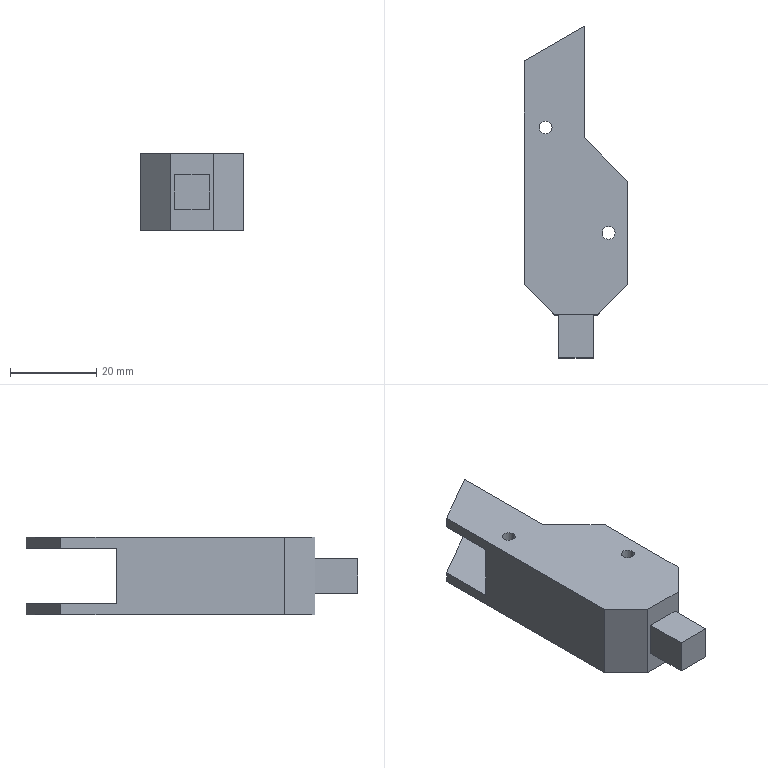Part | SolidWorks | features BaseBody 1 | 1 solid | 33 faces | box 24.142 x 77.176 x 18 mm | volume 8760 mm3 | plane 25 | cylinder 8 | commonest cylinder face diameters 3 x8
STEP:
#1=CARTESIAN_POINT('',(3.5,-15.478,15.5));
#2=VERTEX_POINT('',#1);
#3=CARTESIAN_POINT('',(6.5,-15.478,15.5));
#4=VERTEX_POINT('',#3);
#5=CARTESIAN_POINT('',(5.,-15.478,15.5));
#6=DIRECTION('',(0.,0.,1.));
#7=DIRECTION('',(1.,0.,0.));
#8=AXIS2_PLACEMENT_3D('',#5,#6,#7);
#9=CIRCLE('',#8,1.5);
#10=EDGE_CURVE('',#2,#4,#9,.T.);
#11=ORIENTED_EDGE('',*,*,#10,.F.);
#12=CARTESIAN_POINT('',(3.5,-15.478,18.));
#13=VERTEX_POINT('',#12);
#14=CARTESIAN_POINT('',(3.5,-15.478,-26.));
#15=DIRECTION('',(0.,0.,1.));
#16=VECTOR('',#15,1000.);
#17=LINE('',#14,#16);
#18=EDGE_CURVE('',#2,#13,#17,.T.);
#19=ORIENTED_EDGE('',*,*,#18,.T.);
#20=CARTESIAN_POINT('',(6.5,-15.478,18.));
#21=VERTEX_POINT('',#20);
#22=CARTESIAN_POINT('',(5.,-15.478,18.));
#23=DIRECTION('',(0.,0.,1.));
#24=DIRECTION('',(1.,0.,0.));
#25=AXIS2_PLACEMENT_3D('',#22,#23,#24);
#26=CIRCLE('',#25,1.5);
#27=EDGE_CURVE('',#13,#21,#26,.T.);
#28=ORIENTED_EDGE('',*,*,#27,.T.);
#29=CARTESIAN_POINT('',(6.5,-15.478,-26.));
#30=DIRECTION('',(0.,0.,1.));
#31=VECTOR('',#30,1000.);
#32=LINE('',#29,#31);
#33=EDGE_CURVE('',#4,#21,#32,.T.);
#34=ORIENTED_EDGE('',*,*,#33,.F.);
#35=EDGE_LOOP('',(#11,#19,#28,#34));
#36=FACE_OUTER_BOUND('',#35,.T.);
#37=CARTESIAN_POINT('',(5.,-15.478,-26.));
#38=DIRECTION('',(0.,0.,1.));
#39=DIRECTION('',(1.,0.,0.));
#40=AXIS2_PLACEMENT_3D('',#37,#38,#39);
#41=CYLINDRICAL_SURFACE('',#40,1.5);
#42=ADVANCED_FACE('',(#36),#41,.F.);
#43=CARTESIAN_POINT('',(18.142,-40.,15.5));
#44=VERTEX_POINT('',#43);
#45=CARTESIAN_POINT('',(21.142,-40.,15.5));
#46=VERTEX_POINT('',#45);
#47=CARTESIAN_POINT('',(19.642,-40.,15.5));
#48=DIRECTION('',(0.,0.,1.));
#49=DIRECTION('',(1.,0.,0.));
#50=AXIS2_PLACEMENT_3D('',#47,#48,#49);
#51=CIRCLE('',#50,1.5);
#52=EDGE_CURVE('',#44,#46,#51,.T.);
#53=ORIENTED_EDGE('',*,*,#52,.F.);
#54=CARTESIAN_POINT('',(18.142,-40.,18.));
#55=VERTEX_POINT('',#54);
#56=CARTESIAN_POINT('',(18.142,-40.,-26.));
#57=DIRECTION('',(0.,0.,1.));
#58=VECTOR('',#57,1000.);
#59=LINE('',#56,#58);
#60=EDGE_CURVE('',#44,#55,#59,.T.);
#61=ORIENTED_EDGE('',*,*,#60,.T.);
#62=CARTESIAN_POINT('',(21.142,-40.,18.));
#63=VERTEX_POINT('',#62);
#64=CARTESIAN_POINT('',(19.642,-40.,18.));
#65=DIRECTION('',(0.,0.,1.));
#66=DIRECTION('',(1.,0.,0.));
#67=AXIS2_PLACEMENT_3D('',#64,#65,#66);
#68=CIRCLE('',#67,1.5);
#69=EDGE_CURVE('',#55,#63,#68,.T.);
#70=ORIENTED_EDGE('',*,*,#69,.T.);
#71=CARTESIAN_POINT('',(21.142,-40.,-26.));
#72=DIRECTION('',(0.,0.,1.));
#73=VECTOR('',#72,1000.);
#74=LINE('',#71,#73);
#75=EDGE_CURVE('',#46,#63,#74,.T.);
#76=ORIENTED_EDGE('',*,*,#75,.F.);
#77=EDGE_LOOP('',(#53,#61,#70,#76));
#78=FACE_OUTER_BOUND('',#77,.T.);
#79=CARTESIAN_POINT('',(19.642,-40.,-26.));
#80=DIRECTION('',(0.,0.,1.));
#81=DIRECTION('',(1.,0.,0.));
#82=AXIS2_PLACEMENT_3D('',#79,#80,#81);
#83=CYLINDRICAL_SURFACE('',#82,1.5);
#84=ADVANCED_FACE('',(#78),#83,.F.);
#85=CARTESIAN_POINT('',(3.5,-15.478,0.));
#86=VERTEX_POINT('',#85);
#87=CARTESIAN_POINT('',(6.5,-15.478,0.));
#88=VERTEX_POINT('',#87);
#89=CARTESIAN_POINT('',(5.,-15.478,0.));
#90=DIRECTION('',(0.,0.,1.));
#91=DIRECTION('',(1.,0.,0.));
#92=AXIS2_PLACEMENT_3D('',#89,#90,#91);
#93=CIRCLE('',#92,1.5);
#94=EDGE_CURVE('',#86,#88,#93,.T.);
#95=ORIENTED_EDGE('',*,*,#94,.F.);
#96=CARTESIAN_POINT('',(3.5,-15.478,2.5));
#97=VERTEX_POINT('',#96);
#98=CARTESIAN_POINT('',(3.5,-15.478,-26.));
#99=DIRECTION('',(0.,0.,1.));
#100=VECTOR('',#99,1000.);
#101=LINE('',#98,#100);
#102=EDGE_CURVE('',#86,#97,#101,.T.);
#103=ORIENTED_EDGE('',*,*,#102,.T.);
#104=CARTESIAN_POINT('',(6.5,-15.478,2.5));
#105=VERTEX_POINT('',#104);
#106=CARTESIAN_POINT('',(5.,-15.478,2.5));
#107=DIRECTION('',(0.,0.,1.));
#108=DIRECTION('',(1.,0.,0.));
#109=AXIS2_PLACEMENT_3D('',#106,#107,#108);
#110=CIRCLE('',#109,1.5);
#111=EDGE_CURVE('',#97,#105,#110,.T.);
#112=ORIENTED_EDGE('',*,*,#111,.T.);
#113=CARTESIAN_POINT('',(6.5,-15.478,-26.));
#114=DIRECTION('',(0.,0.,1.));
#115=VECTOR('',#114,1000.);
#116=LINE('',#113,#115);
#117=EDGE_CURVE('',#88,#105,#116,.T.);
#118=ORIENTED_EDGE('',*,*,#117,.F.);
#119=EDGE_LOOP('',(#95,#103,#112,#118));
#120=FACE_OUTER_BOUND('',#119,.T.);
#121=CARTESIAN_POINT('',(5.,-15.478,-26.));
#122=DIRECTION('',(0.,0.,1.));
#123=DIRECTION('',(1.,0.,0.));
#124=AXIS2_PLACEMENT_3D('',#121,#122,#123);
#125=CYLINDRICAL_SURFACE('',#124,1.5);
#126=ADVANCED_FACE('',(#120),#125,.F.);
#127=CARTESIAN_POINT('',(18.142,-40.,0.));
#128=VERTEX_POINT('',#127);
#129=CARTESIAN_POINT('',(21.142,-40.,0.));
#130=VERTEX_POINT('',#129);
#131=CARTESIAN_POINT('',(19.642,-40.,0.));
#132=DIRECTION('',(0.,0.,1.));
#133=DIRECTION('',(1.,0.,0.));
#134=AXIS2_PLACEMENT_3D('',#131,#132,#133);
#135=CIRCLE('',#134,1.5);
#136=EDGE_CURVE('',#128,#130,#135,.T.);
#137=ORIENTED_EDGE('',*,*,#136,.F.);
#138=CARTESIAN_POINT('',(18.142,-40.,2.5));
#139=VERTEX_POINT('',#138);
#140=CARTESIAN_POINT('',(18.142,-40.,-26.));
#141=DIRECTION('',(0.,0.,1.));
#142=VECTOR('',#141,1000.);
#143=LINE('',#140,#142);
#144=EDGE_CURVE('',#128,#139,#143,.T.);
#145=ORIENTED_EDGE('',*,*,#144,.T.);
#146=CARTESIAN_POINT('',(21.142,-40.,2.5));
#147=VERTEX_POINT('',#146);
#148=CARTESIAN_POINT('',(19.642,-40.,2.5));
#149=DIRECTION('',(0.,0.,1.));
#150=DIRECTION('',(1.,0.,0.));
#151=AXIS2_PLACEMENT_3D('',#148,#149,#150);
#152=CIRCLE('',#151,1.5);
#153=EDGE_CURVE('',#139,#147,#152,.T.);
#154=ORIENTED_EDGE('',*,*,#153,.T.);
#155=CARTESIAN_POINT('',(21.142,-40.,-26.));
#156=DIRECTION('',(0.,0.,1.));
#157=VECTOR('',#156,1000.);
#158=LINE('',#155,#157);
#159=EDGE_CURVE('',#130,#147,#158,.T.);
#160=ORIENTED_EDGE('',*,*,#159,.F.);
#161=EDGE_LOOP('',(#137,#145,#154,#160));
#162=FACE_OUTER_BOUND('',#161,.T.);
#163=CARTESIAN_POINT('',(19.642,-40.,-26.));
#164=DIRECTION('',(0.,0.,1.));
#165=DIRECTION('',(1.,0.,0.));
#166=AXIS2_PLACEMENT_3D('',#163,#164,#165);
#167=CYLINDRICAL_SURFACE('',#166,1.5);
#168=ADVANCED_FACE('',(#162),#167,.F.);
#169=CARTESIAN_POINT('',(7.071,-59.071,0.));
#170=VERTEX_POINT('',#169);
#171=CARTESIAN_POINT('',(17.071,-59.071,0.));
#172=VERTEX_POINT('',#171);
#173=CARTESIAN_POINT('',(7.071,-59.071,0.));
#174=DIRECTION('',(1.,0.,0.));
#175=VECTOR('',#174,1000.);
#176=LINE('',#173,#175);
#177=EDGE_CURVE('',#170,#172,#176,.T.);
#178=ORIENTED_EDGE('',*,*,#177,.T.);
#179=CARTESIAN_POINT('',(17.071,-59.071,18.));
#180=VERTEX_POINT('',#179);
#181=CARTESIAN_POINT('',(17.071,-59.071,18.));
#182=DIRECTION('',(0.,0.,-1.));
#183=VECTOR('',#182,1000.);
#184=LINE('',#181,#183);
#185=EDGE_CURVE('',#180,#172,#184,.T.);
#186=ORIENTED_EDGE('',*,*,#185,.F.);
#187=CARTESIAN_POINT('',(7.071,-59.071,18.));
#188=VERTEX_POINT('',#187);
#189=CARTESIAN_POINT('',(7.071,-59.071,18.));
#190=DIRECTION('',(1.,0.,0.));
#191=VECTOR('',#190,1000.);
#192=LINE('',#189,#191);
#193=EDGE_CURVE('',#188,#180,#192,.T.);
#194=ORIENTED_EDGE('',*,*,#193,.F.);
#195=CARTESIAN_POINT('',(7.071,-59.071,18.));
#196=DIRECTION('',(0.,0.,-1.));
#197=VECTOR('',#196,1000.);
#198=LINE('',#195,#197);
#199=EDGE_CURVE('',#188,#170,#198,.T.);
#200=ORIENTED_EDGE('',*,*,#199,.T.);
#201=EDGE_LOOP('',(#178,#186,#194,#200));
#202=FACE_OUTER_BOUND('',#201,.T.);
#203=CARTESIAN_POINT('',(16.071,-59.071,5.));
#204=VERTEX_POINT('',#203);
#205=CARTESIAN_POINT('',(16.071,-59.071,13.));
#206=VERTEX_POINT('',#205);
#207=CARTESIAN_POINT('',(16.071,-59.071,13.));
#208=DIRECTION('',(0.,0.,1.));
#209=VECTOR('',#208,1000.);
#210=LINE('',#207,#209);
#211=EDGE_CURVE('',#204,#206,#210,.T.);
#212=ORIENTED_EDGE('',*,*,#211,.F.);
#213=CARTESIAN_POINT('',(8.071,-59.071,5.));
#214=VERTEX_POINT('',#213);
#215=CARTESIAN_POINT('',(8.071,-59.071,5.));
#216=DIRECTION('',(1.,0.,0.));
#217=VECTOR('',#216,1000.);
#218=LINE('',#215,#217);
#219=EDGE_CURVE('',#214,#204,#218,.T.);
#220=ORIENTED_EDGE('',*,*,#219,.F.);
#221=CARTESIAN_POINT('',(8.071,-59.071,13.));
#222=VERTEX_POINT('',#221);
#223=CARTESIAN_POINT('',(8.071,-59.071,13.));
#224=DIRECTION('',(0.,0.,-1.));
#225=VECTOR('',#224,1000.);
#226=LINE('',#223,#225);
#227=EDGE_CURVE('',#222,#214,#226,.T.);
#228=ORIENTED_EDGE('',*,*,#227,.F.);
#229=CARTESIAN_POINT('',(8.071,-59.071,13.));
#230=DIRECTION('',(-1.,0.,0.));
#231=VECTOR('',#230,1000.);
#232=LINE('',#229,#231);
#233=EDGE_CURVE('',#206,#222,#232,.T.);
#234=ORIENTED_EDGE('',*,*,#233,.F.);
#235=EDGE_LOOP('',(#212,#220,#228,#234));
#236=FACE_BOUND('',#235,.T.);
#237=CARTESIAN_POINT('',(7.071,-59.071,18.));
#238=DIRECTION('',(0.,1.,0.));
#239=DIRECTION('',(0.,0.,1.));
#240=AXIS2_PLACEMENT_3D('',#237,#238,#239);
#241=PLANE('',#240);
#242=ADVANCED_FACE('',(#202,#236),#241,.F.);
#243=CARTESIAN_POINT('',(0.,0.,2.5));
#244=VERTEX_POINT('',#243);
#245=CARTESIAN_POINT('',(0.,0.,0.));
#246=VERTEX_POINT('',#245);
#247=CARTESIAN_POINT('',(0.,0.,18.));
#248=DIRECTION('',(0.,0.,-1.));
#249=VECTOR('',#248,1000.);
#250=LINE('',#247,#249);
#251=EDGE_CURVE('',#244,#246,#250,.T.);
#252=ORIENTED_EDGE('',*,*,#251,.F.);
#253=CARTESIAN_POINT('',(14.038,8.105,2.5));
#254=VERTEX_POINT('',#253);
#255=CARTESIAN_POINT('',(14.038,8.105,2.5));
#256=DIRECTION('',(-0.866,-0.5,0.));
#257=VECTOR('',#256,1000.);
#258=LINE('',#255,#257);
#259=EDGE_CURVE('',#254,#244,#258,.T.);
#260=ORIENTED_EDGE('',*,*,#259,.F.);
#261=CARTESIAN_POINT('',(14.038,8.105,0.));
#262=VERTEX_POINT('',#261);
#263=CARTESIAN_POINT('',(14.038,8.105,18.));
#264=DIRECTION('',(0.,0.,-1.));
#265=VECTOR('',#264,1000.);
#266=LINE('',#263,#265);
#267=EDGE_CURVE('',#254,#262,#266,.T.);
#268=ORIENTED_EDGE('',*,*,#267,.T.);
#269=CARTESIAN_POINT('',(14.038,8.105,0.));
#270=DIRECTION('',(-0.866,-0.5,0.));
#271=VECTOR('',#270,1000.);
#272=LINE('',#269,#271);
#273=EDGE_CURVE('',#262,#246,#272,.T.);
#274=ORIENTED_EDGE('',*,*,#273,.T.);
#275=EDGE_LOOP('',(#252,#260,#268,#274));
#276=FACE_OUTER_BOUND('',#275,.T.);
#277=CARTESIAN_POINT('',(14.038,8.105,18.));
#278=DIRECTION('',(0.5,-0.866,0.));
#279=DIRECTION('',(0.866,0.5,0.));
#280=AXIS2_PLACEMENT_3D('',#277,#278,#279);
#281=PLANE('',#280);
#282=ADVANCED_FACE('',(#276),#281,.F.);
#283=CARTESIAN_POINT('',(14.038,8.105,15.5));
#284=VERTEX_POINT('',#283);
#285=CARTESIAN_POINT('',(0.,0.,15.5));
#286=VERTEX_POINT('',#285);
#287=CARTESIAN_POINT('',(14.038,8.105,15.5));
#288=DIRECTION('',(-0.866,-0.5,0.));
#289=VECTOR('',#288,1000.);
#290=LINE('',#287,#289);
#291=EDGE_CURVE('',#284,#286,#290,.T.);
#292=ORIENTED_EDGE('',*,*,#291,.T.);
#293=CARTESIAN_POINT('',(0.,0.,18.));
#294=VERTEX_POINT('',#293);
#295=CARTESIAN_POINT('',(0.,0.,18.));
#296=DIRECTION('',(0.,0.,-1.));
#297=VECTOR('',#296,1000.);
#298=LINE('',#295,#297);
#299=EDGE_CURVE('',#294,#286,#298,.T.);
#300=ORIENTED_EDGE('',*,*,#299,.F.);
#301=CARTESIAN_POINT('',(14.038,8.105,18.));
#302=VERTEX_POINT('',#301);
#303=CARTESIAN_POINT('',(14.038,8.105,18.));
#304=DIRECTION('',(-0.866,-0.5,0.));
#305=VECTOR('',#304,1000.);
#306=LINE('',#303,#305);
#307=EDGE_CURVE('',#302,#294,#306,.T.);
#308=ORIENTED_EDGE('',*,*,#307,.F.);
#309=CARTESIAN_POINT('',(14.038,8.105,18.));
#310=DIRECTION('',(0.,0.,-1.));
#311=VECTOR('',#310,1000.);
#312=LINE('',#309,#311);
#313=EDGE_CURVE('',#302,#284,#312,.T.);
#314=ORIENTED_EDGE('',*,*,#313,.T.);
#315=EDGE_LOOP('',(#292,#300,#308,#314));
#316=FACE_OUTER_BOUND('',#315,.T.);
#317=CARTESIAN_POINT('',(14.038,8.105,18.));
#318=DIRECTION('',(0.5,-0.866,0.));
#319=DIRECTION('',(0.866,0.5,0.));
#320=AXIS2_PLACEMENT_3D('',#317,#318,#319);
#321=PLANE('',#320);
#322=ADVANCED_FACE('',(#316),#321,.F.);
#323=CARTESIAN_POINT('',(24.142,-48.464,2.5));
#324=VERTEX_POINT('',#323);
#325=CARTESIAN_POINT('',(24.142,-28.,2.5));
#326=VERTEX_POINT('',#325);
#327=CARTESIAN_POINT('',(24.142,-52.,2.5));
#328=DIRECTION('',(0.,1.,0.));
#329=VECTOR('',#328,1000.);
#330=LINE('',#327,#329);
#331=EDGE_CURVE('',#324,#326,#330,.T.);
#332=ORIENTED_EDGE('',*,*,#331,.F.);
#333=CARTESIAN_POINT('',(24.142,-48.464,15.5));
#334=VERTEX_POINT('',#333);
#335=CARTESIAN_POINT('',(24.142,-48.464,18.));
#336=DIRECTION('',(0.,0.,-1.));
#337=VECTOR('',#336,1000.);
#338=LINE('',#335,#337);
#339=EDGE_CURVE('',#334,#324,#338,.T.);
#340=ORIENTED_EDGE('',*,*,#339,.F.);
#341=CARTESIAN_POINT('',(24.142,-28.,15.5));
#342=VERTEX_POINT('',#341);
#343=CARTESIAN_POINT('',(24.142,-52.,15.5));
#344=DIRECTION('',(0.,1.,0.));
#345=VECTOR('',#344,1000.);
#346=LINE('',#343,#345);
#347=EDGE_CURVE('',#334,#342,#346,.T.);
#348=ORIENTED_EDGE('',*,*,#347,.T.);
#349=CARTESIAN_POINT('',(24.142,-28.,18.));
#350=VERTEX_POINT('',#349);
#351=CARTESIAN_POINT('',(24.142,-28.,18.));
#352=DIRECTION('',(0.,0.,-1.));
#353=VECTOR('',#352,1000.);
#354=LINE('',#351,#353);
#355=EDGE_CURVE('',#350,#342,#354,.T.);
#356=ORIENTED_EDGE('',*,*,#355,.F.);
#357=CARTESIAN_POINT('',(24.142,-52.,18.));
#358=VERTEX_POINT('',#357);
#359=CARTESIAN_POINT('',(24.142,-52.,18.));
#360=DIRECTION('',(0.,1.,0.));
#361=VECTOR('',#360,1000.);
#362=LINE('',#359,#361);
#363=EDGE_CURVE('',#358,#350,#362,.T.);
#364=ORIENTED_EDGE('',*,*,#363,.F.);
#365=CARTESIAN_POINT('',(24.142,-52.,0.));
#366=VERTEX_POINT('',#365);
#367=CARTESIAN_POINT('',(24.142,-52.,18.));
#368=DIRECTION('',(0.,0.,-1.));
#369=VECTOR('',#368,1000.);
#370=LINE('',#367,#369);
#371=EDGE_CURVE('',#358,#366,#370,.T.);
#372=ORIENTED_EDGE('',*,*,#371,.T.);
#373=CARTESIAN_POINT('',(24.142,-28.,0.));
#374=VERTEX_POINT('',#373);
#375=CARTESIAN_POINT('',(24.142,-52.,0.));
#376=DIRECTION('',(0.,1.,0.));
#377=VECTOR('',#376,1000.);
#378=LINE('',#375,#377);
#379=EDGE_CURVE('',#366,#374,#378,.T.);
#380=ORIENTED_EDGE('',*,*,#379,.T.);
#381=CARTESIAN_POINT('',(24.142,-28.,18.));
#382=DIRECTION('',(0.,0.,-1.));
#383=VECTOR('',#382,1000.);
#384=LINE('',#381,#383);
#385=EDGE_CURVE('',#326,#374,#384,.T.);
#386=ORIENTED_EDGE('',*,*,#385,.F.);
#387=EDGE_LOOP('',(#332,#340,#348,#356,#364,#372,#380,#386));
#388=FACE_OUTER_BOUND('',#387,.T.);
#389=CARTESIAN_POINT('',(24.142,-52.,18.));
#390=DIRECTION('',(-1.,0.,0.));
#391=DIRECTION('',(0.,0.,1.));
#392=AXIS2_PLACEMENT_3D('',#389,#390,#391);
#393=PLANE('',#392);
#394=ADVANCED_FACE('',(#388),#393,.F.);
#395=CARTESIAN_POINT('',(14.038,-17.895,2.5));
#396=VERTEX_POINT('',#395);
#397=CARTESIAN_POINT('',(24.142,-28.,2.5));
#398=DIRECTION('',(-0.7071,0.7071,0.));
#399=VECTOR('',#398,1000.);
#400=LINE('',#397,#399);
#401=EDGE_CURVE('',#326,#396,#400,.T.);
#402=ORIENTED_EDGE('',*,*,#401,.F.);
#403=ORIENTED_EDGE('',*,*,#385,.T.);
#404=CARTESIAN_POINT('',(14.038,-17.895,0.));
#405=VERTEX_POINT('',#404);
#406=CARTESIAN_POINT('',(24.142,-28.,0.));
#407=DIRECTION('',(-0.7071,0.7071,0.));
#408=VECTOR('',#407,1000.);
#409=LINE('',#406,#408);
#410=EDGE_CURVE('',#374,#405,#409,.T.);
#411=ORIENTED_EDGE('',*,*,#410,.T.);
#412=CARTESIAN_POINT('',(14.038,-17.895,18.));
#413=DIRECTION('',(0.,0.,-1.));
#414=VECTOR('',#413,1000.);
#415=LINE('',#412,#414);
#416=EDGE_CURVE('',#396,#405,#415,.T.);
#417=ORIENTED_EDGE('',*,*,#416,.F.);
#418=EDGE_LOOP('',(#402,#403,#411,#417));
#419=FACE_OUTER_BOUND('',#418,.T.);
#420=CARTESIAN_POINT('',(24.142,-28.,18.));
#421=DIRECTION('',(-0.7071,-0.7071,0.));
#422=DIRECTION('',(0.7071,-0.7071,0.));
#423=AXIS2_PLACEMENT_3D('',#420,#421,#422);
#424=PLANE('',#423);
#425=ADVANCED_FACE('',(#419),#424,.F.);
#426=CARTESIAN_POINT('',(14.038,-17.895,2.5));
#427=DIRECTION('',(0.,1.,0.));
#428=VECTOR('',#427,1000.);
#429=LINE('',#426,#428);
#430=EDGE_CURVE('',#396,#254,#429,.T.);
#431=ORIENTED_EDGE('',*,*,#430,.F.);
#432=ORIENTED_EDGE('',*,*,#416,.T.);
#433=CARTESIAN_POINT('',(14.038,-17.895,0.));
#434=DIRECTION('',(0.,1.,0.));
#435=VECTOR('',#434,1000.);
#436=LINE('',#433,#435);
#437=EDGE_CURVE('',#405,#262,#436,.T.);
#438=ORIENTED_EDGE('',*,*,#437,.T.);
#439=ORIENTED_EDGE('',*,*,#267,.F.);
#440=EDGE_LOOP('',(#431,#432,#438,#439));
#441=FACE_OUTER_BOUND('',#440,.T.);
#442=CARTESIAN_POINT('',(14.038,-17.895,18.));
#443=DIRECTION('',(-1.,0.,0.));
#444=DIRECTION('',(0.,-1.,0.));
#445=AXIS2_PLACEMENT_3D('',#442,#443,#444);
#446=PLANE('',#445);
#447=ADVANCED_FACE('',(#441),#446,.F.);
#448=CARTESIAN_POINT('',(0.,-12.895,2.5));
#449=VERTEX_POINT('',#448);
#450=CARTESIAN_POINT('',(0.,-12.895,15.5));
#451=VERTEX_POINT('',#450);
#452=CARTESIAN_POINT('',(0.,-12.895,2.5));
#453=DIRECTION('',(0.,0.,1.));
#454=VECTOR('',#453,1000.);
#455=LINE('',#452,#454);
#456=EDGE_CURVE('',#449,#451,#455,.T.);
#457=ORIENTED_EDGE('',*,*,#456,.F.);
#458=CARTESIAN_POINT('',(0.,8.105,2.5));
#459=DIRECTION('',(0.,-1.,0.));
#460=VECTOR('',#459,1000.);
#461=LINE('',#458,#460);
#462=EDGE_CURVE('',#244,#449,#461,.T.);
#463=ORIENTED_EDGE('',*,*,#462,.F.);
#464=ORIENTED_EDGE('',*,*,#251,.T.);
#465=CARTESIAN_POINT('',(0.,-52.,0.));
#466=VERTEX_POINT('',#465);
#467=CARTESIAN_POINT('',(0.,0.,0.));
#468=DIRECTION('',(0.,-1.,0.));
#469=VECTOR('',#468,1000.);
#470=LINE('',#467,#469);
#471=EDGE_CURVE('',#246,#466,#470,.T.);
#472=ORIENTED_EDGE('',*,*,#471,.T.);
#473=CARTESIAN_POINT('',(0.,-52.,18.));
#474=VERTEX_POINT('',#473);
#475=CARTESIAN_POINT('',(0.,-52.,18.));
#476=DIRECTION('',(0.,0.,-1.));
#477=VECTOR('',#476,1000.);
#478=LINE('',#475,#477);
#479=EDGE_CURVE('',#474,#466,#478,.T.);
#480=ORIENTED_EDGE('',*,*,#479,.F.);
#481=CARTESIAN_POINT('',(0.,0.,18.));
#482=DIRECTION('',(0.,-1.,0.));
#483=VECTOR('',#482,1000.);
#484=LINE('',#481,#483);
#485=EDGE_CURVE('',#294,#474,#484,.T.);
#486=ORIENTED_EDGE('',*,*,#485,.F.);
#487=ORIENTED_EDGE('',*,*,#299,.T.);
#488=CARTESIAN_POINT('',(0.,8.105,15.5));
#489=DIRECTION('',(0.,1.,0.));
#490=VECTOR('',#489,1000.);
#491=LINE('',#488,#490);
#492=EDGE_CURVE('',#451,#286,#491,.T.);
#493=ORIENTED_EDGE('',*,*,#492,.F.);
#494=EDGE_LOOP('',(#457,#463,#464,#472,#480,#486,#487,#493));
#495=FACE_OUTER_BOUND('',#494,.T.);
#496=CARTESIAN_POINT('',(0.,0.,18.));
#497=DIRECTION('',(1.,0.,0.));
#498=DIRECTION('',(0.,1.,0.));
#499=AXIS2_PLACEMENT_3D('',#496,#497,#498);
#500=PLANE('',#499);
#501=ADVANCED_FACE('',(#495),#500,.F.);
#502=CARTESIAN_POINT('',(0.,-52.,0.));
#503=DIRECTION('',(0.7071,-0.7071,0.));
#504=VECTOR('',#503,1000.);
#505=LINE('',#502,#504);
#506=EDGE_CURVE('',#466,#170,#505,.T.);
#507=ORIENTED_EDGE('',*,*,#506,.T.);
#508=ORIENTED_EDGE('',*,*,#199,.F.);
#509=CARTESIAN_POINT('',(0.,-52.,18.));
#510=DIRECTION('',(0.7071,-0.7071,0.));
#511=VECTOR('',#510,1000.);
#512=LINE('',#509,#511);
#513=EDGE_CURVE('',#474,#188,#512,.T.);
#514=ORIENTED_EDGE('',*,*,#513,.F.);
#515=ORIENTED_EDGE('',*,*,#479,.T.);
#516=EDGE_LOOP('',(#507,#508,#514,#515));
#517=FACE_OUTER_BOUND('',#516,.T.);
#518=CARTESIAN_POINT('',(0.,-52.,18.));
#519=DIRECTION('',(0.7071,0.7071,0.));
#520=DIRECTION('',(-0.7071,0.7071,0.));
#521=AXIS2_PLACEMENT_3D('',#518,#519,#520);
#522=PLANE('',#521);
#523=ADVANCED_FACE('',(#517),#522,.F.);
#524=CARTESIAN_POINT('',(17.071,-59.071,0.));
#525=DIRECTION('',(0.7071,0.7071,0.));
#526=VECTOR('',#525,1000.);
#527=LINE('',#524,#526);
#528=EDGE_CURVE('',#172,#366,#527,.T.);
#529=ORIENTED_EDGE('',*,*,#528,.T.);
#530=ORIENTED_EDGE('',*,*,#371,.F.);
#531=CARTESIAN_POINT('',(17.071,-59.071,18.));
#532=DIRECTION('',(0.7071,0.7071,0.));
#533=VECTOR('',#532,1000.);
#534=LINE('',#531,#533);
#535=EDGE_CURVE('',#180,#358,#534,.T.);
#536=ORIENTED_EDGE('',*,*,#535,.F.);
#537=ORIENTED_EDGE('',*,*,#185,.T.);
#538=EDGE_LOOP('',(#529,#530,#536,#537));
#539=FACE_OUTER_BOUND('',#538,.T.);
#540=CARTESIAN_POINT('',(17.071,-59.071,18.));
#541=DIRECTION('',(-0.7071,0.7071,0.));
#542=DIRECTION('',(-0.7071,-0.7071,0.));
#543=AXIS2_PLACEMENT_3D('',#540,#541,#542);
#544=PLANE('',#543);
#545=ADVANCED_FACE('',(#539),#544,.F.);
#546=ORIENTED_EDGE('',*,*,#355,.T.);
#547=CARTESIAN_POINT('',(14.038,-17.895,15.5));
#548=VERTEX_POINT('',#547);
#549=CARTESIAN_POINT('',(24.142,-28.,15.5));
#550=DIRECTION('',(-0.7071,0.7071,0.));
#551=VECTOR('',#550,1000.);
#552=LINE('',#549,#551);
#553=EDGE_CURVE('',#342,#548,#552,.T.);
#554=ORIENTED_EDGE('',*,*,#553,.T.);
#555=CARTESIAN_POINT('',(14.038,-17.895,18.));
#556=VERTEX_POINT('',#555);
#557=CARTESIAN_POINT('',(14.038,-17.895,18.));
#558=DIRECTION('',(0.,0.,-1.));
#559=VECTOR('',#558,1000.);
#560=LINE('',#557,#559);
#561=EDGE_CURVE('',#556,#548,#560,.T.);
#562=ORIENTED_EDGE('',*,*,#561,.F.);
#563=CARTESIAN_POINT('',(24.142,-28.,18.));
#564=DIRECTION('',(-0.7071,0.7071,0.));
#565=VECTOR('',#564,1000.);
#566=LINE('',#563,#565);
#567=EDGE_CURVE('',#350,#556,#566,.T.);
#568=ORIENTED_EDGE('',*,*,#567,.F.);
#569=EDGE_LOOP('',(#546,#554,#562,#568));
#570=FACE_OUTER_BOUND('',#569,.T.);
#571=CARTESIAN_POINT('',(24.142,-28.,18.));
#572=DIRECTION('',(-0.7071,-0.7071,0.));
#573=DIRECTION('',(0.7071,-0.7071,0.));
#574=AXIS2_PLACEMENT_3D('',#571,#572,#573);
#575=PLANE('',#574);
#576=ADVANCED_FACE('',(#570),#575,.F.);
#577=ORIENTED_EDGE('',*,*,#561,.T.);
#578=CARTESIAN_POINT('',(14.038,-17.895,15.5));
#579=DIRECTION('',(0.,1.,0.));
#580=VECTOR('',#579,1000.);
#581=LINE('',#578,#580);
#582=EDGE_CURVE('',#548,#284,#581,.T.);
#583=ORIENTED_EDGE('',*,*,#582,.T.);
#584=ORIENTED_EDGE('',*,*,#313,.F.);
#585=CARTESIAN_POINT('',(14.038,-17.895,18.));
#586=DIRECTION('',(0.,1.,0.));
#587=VECTOR('',#586,1000.);
#588=LINE('',#585,#587);
#589=EDGE_CURVE('',#556,#302,#588,.T.);
#590=ORIENTED_EDGE('',*,*,#589,.F.);
#591=EDGE_LOOP('',(#577,#583,#584,#590));
#592=FACE_OUTER_BOUND('',#591,.T.);
#593=CARTESIAN_POINT('',(14.038,-17.895,18.));
#594=DIRECTION('',(-1.,0.,0.));
#595=DIRECTION('',(0.,-1.,0.));
#596=AXIS2_PLACEMENT_3D('',#593,#594,#595);
#597=PLANE('',#596);
#598=ADVANCED_FACE('',(#592),#597,.F.);
#599=CARTESIAN_POINT('',(5.,-15.478,18.));
#600=DIRECTION('',(0.,0.,1.));
#601=DIRECTION('',(1.,0.,0.));
#602=AXIS2_PLACEMENT_3D('',#599,#600,#601);
#603=CIRCLE('',#602,1.5);
#604=EDGE_CURVE('',#21,#13,#603,.T.);
#605=ORIENTED_EDGE('',*,*,#604,.F.);
#606=ORIENTED_EDGE('',*,*,#27,.F.);
#607=EDGE_LOOP('',(#605,#606));
#608=FACE_BOUND('',#607,.T.);
#609=CARTESIAN_POINT('',(19.642,-40.,18.));
#610=DIRECTION('',(0.,0.,1.));
#611=DIRECTION('',(1.,0.,0.));
#612=AXIS2_PLACEMENT_3D('',#609,#610,#611);
#613=CIRCLE('',#612,1.5);
#614=EDGE_CURVE('',#63,#55,#613,.T.);
#615=ORIENTED_EDGE('',*,*,#614,.F.);
#616=ORIENTED_EDGE('',*,*,#69,.F.);
#617=EDGE_LOOP('',(#615,#616));
#618=FACE_BOUND('',#617,.T.);
#619=ORIENTED_EDGE('',*,*,#307,.T.);
#620=ORIENTED_EDGE('',*,*,#485,.T.);
#621=ORIENTED_EDGE('',*,*,#513,.T.);
#622=ORIENTED_EDGE('',*,*,#193,.T.);
#623=ORIENTED_EDGE('',*,*,#535,.T.);
#624=ORIENTED_EDGE('',*,*,#363,.T.);
#625=ORIENTED_EDGE('',*,*,#567,.T.);
#626=ORIENTED_EDGE('',*,*,#589,.T.);
#627=EDGE_LOOP('',(#619,#620,#621,#622,#623,#624,#625,#626));
#628=FACE_OUTER_BOUND('',#627,.T.);
#629=CARTESIAN_POINT('',(0.,0.,18.));
#630=DIRECTION('',(0.,0.,1.));
#631=DIRECTION('',(1.,0.,0.));
#632=AXIS2_PLACEMENT_3D('',#629,#630,#631);
#633=PLANE('',#632);
#634=ADVANCED_FACE('',(#608,#618,#628),#633,.T.);
#635=CARTESIAN_POINT('',(5.,-15.478,0.));
#636=DIRECTION('',(0.,0.,1.));
#637=DIRECTION('',(1.,0.,0.));
#638=AXIS2_PLACEMENT_3D('',#635,#636,#637);
#639=CIRCLE('',#638,1.5);
#640=EDGE_CURVE('',#88,#86,#639,.T.);
#641=ORIENTED_EDGE('',*,*,#640,.T.);
#642=ORIENTED_EDGE('',*,*,#94,.T.);
#643=EDGE_LOOP('',(#641,#642));
#644=FACE_BOUND('',#643,.T.);
#645=CARTESIAN_POINT('',(19.642,-40.,0.));
#646=DIRECTION('',(0.,0.,1.));
#647=DIRECTION('',(1.,0.,0.));
#648=AXIS2_PLACEMENT_3D('',#645,#646,#647);
#649=CIRCLE('',#648,1.5);
#650=EDGE_CURVE('',#130,#128,#649,.T.);
#651=ORIENTED_EDGE('',*,*,#650,.T.);
#652=ORIENTED_EDGE('',*,*,#136,.T.);
#653=EDGE_LOOP('',(#651,#652));
#654=FACE_BOUND('',#653,.T.);
#655=ORIENTED_EDGE('',*,*,#273,.F.);
#656=ORIENTED_EDGE('',*,*,#437,.F.);
#657=ORIENTED_EDGE('',*,*,#410,.F.);
#658=ORIENTED_EDGE('',*,*,#379,.F.);
#659=ORIENTED_EDGE('',*,*,#528,.F.);
#660=ORIENTED_EDGE('',*,*,#177,.F.);
#661=ORIENTED_EDGE('',*,*,#506,.F.);
#662=ORIENTED_EDGE('',*,*,#471,.F.);
#663=EDGE_LOOP('',(#655,#656,#657,#658,#659,#660,#661,#662));
#664=FACE_OUTER_BOUND('',#663,.T.);
#665=CARTESIAN_POINT('',(0.,0.,0.));
#666=DIRECTION('',(0.,0.,1.));
#667=DIRECTION('',(1.,0.,0.));
#668=AXIS2_PLACEMENT_3D('',#665,#666,#667);
#669=PLANE('',#668);
#670=ADVANCED_FACE('',(#644,#654,#664),#669,.F.);
#671=CARTESIAN_POINT('',(2.5,-12.895,15.5));
#672=VERTEX_POINT('',#671);
#673=CARTESIAN_POINT('',(2.5,-12.895,2.5));
#674=VERTEX_POINT('',#673);
#675=CARTESIAN_POINT('',(2.5,-12.895,18.));
#676=DIRECTION('',(0.,0.,-1.));
#677=VECTOR('',#676,1000.);
#678=LINE('',#675,#677);
#679=EDGE_CURVE('',#672,#674,#678,.T.);
#680=ORIENTED_EDGE('',*,*,#679,.F.);
#681=CARTESIAN_POINT('',(2.5,-50.964,15.5));
#682=VERTEX_POINT('',#681);
#683=CARTESIAN_POINT('',(2.5,0.,15.5));
#684=DIRECTION('',(0.,-1.,0.));
#685=VECTOR('',#684,1000.);
#686=LINE('',#683,#685);
#687=EDGE_CURVE('',#672,#682,#686,.T.);
#688=ORIENTED_EDGE('',*,*,#687,.T.);
#689=CARTESIAN_POINT('',(2.5,-50.964,2.5));
#690=VERTEX_POINT('',#689);
#691=CARTESIAN_POINT('',(2.5,-50.964,18.));
#692=DIRECTION('',(0.,0.,-1.));
#693=VECTOR('',#692,1000.);
#694=LINE('',#691,#693);
#695=EDGE_CURVE('',#682,#690,#694,.T.);
#696=ORIENTED_EDGE('',*,*,#695,.T.);
#697=CARTESIAN_POINT('',(2.5,0.,2.5));
#698=DIRECTION('',(0.,-1.,0.));
#699=VECTOR('',#698,1000.);
#700=LINE('',#697,#699);
#701=EDGE_CURVE('',#674,#690,#700,.T.);
#702=ORIENTED_EDGE('',*,*,#701,.F.);
#703=EDGE_LOOP('',(#680,#688,#696,#702));
#704=FACE_OUTER_BOUND('',#703,.T.);
#705=CARTESIAN_POINT('',(2.5,0.,18.));
#706=DIRECTION('',(1.,0.,0.));
#707=DIRECTION('',(0.,1.,0.));
#708=AXIS2_PLACEMENT_3D('',#705,#706,#707);
#709=PLANE('',#708);
#710=ADVANCED_FACE('',(#704),#709,.T.);
#711=CARTESIAN_POINT('',(8.107,-56.571,2.5));
#712=VERTEX_POINT('',#711);
#713=CARTESIAN_POINT('',(1.768,-50.232,2.5));
#714=DIRECTION('',(0.7071,-0.7071,0.));
#715=VECTOR('',#714,1000.);
#716=LINE('',#713,#715);
#717=EDGE_CURVE('',#690,#712,#716,.T.);
#718=ORIENTED_EDGE('',*,*,#717,.F.);
#719=ORIENTED_EDGE('',*,*,#695,.F.);
#720=CARTESIAN_POINT('',(8.107,-56.571,15.5));
#721=VERTEX_POINT('',#720);
#722=CARTESIAN_POINT('',(1.768,-50.232,15.5));
#723=DIRECTION('',(0.7071,-0.7071,0.));
#724=VECTOR('',#723,1000.);
#725=LINE('',#722,#724);
#726=EDGE_CURVE('',#682,#721,#725,.T.);
#727=ORIENTED_EDGE('',*,*,#726,.T.);
#728=CARTESIAN_POINT('',(8.107,-56.571,18.));
#729=DIRECTION('',(0.,0.,-1.));
#730=VECTOR('',#729,1000.);
#731=LINE('',#728,#730);
#732=EDGE_CURVE('',#721,#712,#731,.T.);
#733=ORIENTED_EDGE('',*,*,#732,.T.);
#734=EDGE_LOOP('',(#718,#719,#727,#733));
#735=FACE_OUTER_BOUND('',#734,.T.);
#736=CARTESIAN_POINT('',(1.768,-50.232,18.));
#737=DIRECTION('',(0.7071,0.7071,0.));
#738=DIRECTION('',(-0.7071,0.7071,0.));
#739=AXIS2_PLACEMENT_3D('',#736,#737,#738);
#740=PLANE('',#739);
#741=ADVANCED_FACE('',(#735),#740,.T.);
#742=CARTESIAN_POINT('',(16.036,-56.571,2.5));
#743=VERTEX_POINT('',#742);
#744=CARTESIAN_POINT('',(7.071,-56.571,2.5));
#745=DIRECTION('',(1.,0.,0.));
#746=VECTOR('',#745,1000.);
#747=LINE('',#744,#746);
#748=EDGE_CURVE('',#712,#743,#747,.T.);
#749=ORIENTED_EDGE('',*,*,#748,.F.);
#750=ORIENTED_EDGE('',*,*,#732,.F.);
#751=CARTESIAN_POINT('',(16.036,-56.571,15.5));
#752=VERTEX_POINT('',#751);
#753=CARTESIAN_POINT('',(7.071,-56.571,15.5));
#754=DIRECTION('',(1.,0.,0.));
#755=VECTOR('',#754,1000.);
#756=LINE('',#753,#755);
#757=EDGE_CURVE('',#721,#752,#756,.T.);
#758=ORIENTED_EDGE('',*,*,#757,.T.);
#759=CARTESIAN_POINT('',(16.036,-56.571,18.));
#760=DIRECTION('',(0.,0.,-1.));
#761=VECTOR('',#760,1000.);
#762=LINE('',#759,#761);
#763=EDGE_CURVE('',#752,#743,#762,.T.);
#764=ORIENTED_EDGE('',*,*,#763,.T.);
#765=EDGE_LOOP('',(#749,#750,#758,#764));
#766=FACE_OUTER_BOUND('',#765,.T.);
#767=CARTESIAN_POINT('',(7.071,-56.571,18.));
#768=DIRECTION('',(0.,1.,0.));
#769=DIRECTION('',(0.,0.,1.));
#770=AXIS2_PLACEMENT_3D('',#767,#768,#769);
#771=PLANE('',#770);
#772=ADVANCED_FACE('',(#766),#771,.T.);
#773=CARTESIAN_POINT('',(15.303,-57.303,2.5));
#774=DIRECTION('',(0.7071,0.7071,0.));
#775=VECTOR('',#774,1000.);
#776=LINE('',#773,#775);
#777=EDGE_CURVE('',#743,#324,#776,.T.);
#778=ORIENTED_EDGE('',*,*,#777,.F.);
#779=ORIENTED_EDGE('',*,*,#763,.F.);
#780=CARTESIAN_POINT('',(15.303,-57.303,15.5));
#781=DIRECTION('',(0.7071,0.7071,0.));
#782=VECTOR('',#781,1000.);
#783=LINE('',#780,#782);
#784=EDGE_CURVE('',#752,#334,#783,.T.);
#785=ORIENTED_EDGE('',*,*,#784,.T.);
#786=ORIENTED_EDGE('',*,*,#339,.T.);
#787=EDGE_LOOP('',(#778,#779,#785,#786));
#788=FACE_OUTER_BOUND('',#787,.T.);
#789=CARTESIAN_POINT('',(15.303,-57.303,18.));
#790=DIRECTION('',(-0.7071,0.7071,0.));
#791=DIRECTION('',(-0.7071,-0.7071,0.));
#792=AXIS2_PLACEMENT_3D('',#789,#790,#791);
#793=PLANE('',#792);
#794=ADVANCED_FACE('',(#788),#793,.T.);
#795=CARTESIAN_POINT('',(5.,-15.478,15.5));
#796=DIRECTION('',(0.,0.,1.));
#797=DIRECTION('',(1.,0.,0.));
#798=AXIS2_PLACEMENT_3D('',#795,#796,#797);
#799=CIRCLE('',#798,1.5);
#800=EDGE_CURVE('',#4,#2,#799,.T.);
#801=ORIENTED_EDGE('',*,*,#800,.T.);
#802=ORIENTED_EDGE('',*,*,#10,.T.);
#803=EDGE_LOOP('',(#801,#802));
#804=FACE_BOUND('',#803,.T.);
#805=CARTESIAN_POINT('',(19.642,-40.,15.5));
#806=DIRECTION('',(0.,0.,1.));
#807=DIRECTION('',(1.,0.,0.));
#808=AXIS2_PLACEMENT_3D('',#805,#806,#807);
#809=CIRCLE('',#808,1.5);
#810=EDGE_CURVE('',#46,#44,#809,.T.);
#811=ORIENTED_EDGE('',*,*,#810,.T.);
#812=ORIENTED_EDGE('',*,*,#52,.T.);
#813=EDGE_LOOP('',(#811,#812));
#814=FACE_BOUND('',#813,.T.);
#815=ORIENTED_EDGE('',*,*,#687,.F.);
#816=CARTESIAN_POINT('',(44.,-12.895,15.5));
#817=DIRECTION('',(-1.,0.,0.));
#818=VECTOR('',#817,1000.);
#819=LINE('',#816,#818);
#820=EDGE_CURVE('',#672,#451,#819,.T.);
#821=ORIENTED_EDGE('',*,*,#820,.T.);
#822=ORIENTED_EDGE('',*,*,#492,.T.);
#823=ORIENTED_EDGE('',*,*,#291,.F.);
#824=ORIENTED_EDGE('',*,*,#582,.F.);
#825=ORIENTED_EDGE('',*,*,#553,.F.);
#826=ORIENTED_EDGE('',*,*,#347,.F.);
#827=ORIENTED_EDGE('',*,*,#784,.F.);
#828=ORIENTED_EDGE('',*,*,#757,.F.);
#829=ORIENTED_EDGE('',*,*,#726,.F.);
#830=EDGE_LOOP('',(#815,#821,#822,#823,#824,#825,#826,#827,#828,#829));
#831=FACE_OUTER_BOUND('',#830,.T.);
#832=CARTESIAN_POINT('',(0.,0.,15.5));
#833=DIRECTION('',(0.,0.,1.));
#834=DIRECTION('',(1.,0.,0.));
#835=AXIS2_PLACEMENT_3D('',#832,#833,#834);
#836=PLANE('',#835);
#837=ADVANCED_FACE('',(#804,#814,#831),#836,.F.);
#838=CARTESIAN_POINT('',(5.,-15.478,2.5));
#839=DIRECTION('',(0.,0.,1.));
#840=DIRECTION('',(1.,0.,0.));
#841=AXIS2_PLACEMENT_3D('',#838,#839,#840);
#842=CIRCLE('',#841,1.5);
#843=EDGE_CURVE('',#105,#97,#842,.T.);
#844=ORIENTED_EDGE('',*,*,#843,.F.);
#845=ORIENTED_EDGE('',*,*,#111,.F.);
#846=EDGE_LOOP('',(#844,#845));
#847=FACE_BOUND('',#846,.T.);
#848=CARTESIAN_POINT('',(19.642,-40.,2.5));
#849=DIRECTION('',(0.,0.,1.));
#850=DIRECTION('',(1.,0.,0.));
#851=AXIS2_PLACEMENT_3D('',#848,#849,#850);
#852=CIRCLE('',#851,1.5);
#853=EDGE_CURVE('',#147,#139,#852,.T.);
#854=ORIENTED_EDGE('',*,*,#853,.F.);
#855=ORIENTED_EDGE('',*,*,#153,.F.);
#856=EDGE_LOOP('',(#854,#855));
#857=FACE_BOUND('',#856,.T.);
#858=ORIENTED_EDGE('',*,*,#430,.T.);
#859=ORIENTED_EDGE('',*,*,#259,.T.);
#860=ORIENTED_EDGE('',*,*,#462,.T.);
#861=CARTESIAN_POINT('',(44.,-12.895,2.5));
#862=DIRECTION('',(-1.,0.,0.));
#863=VECTOR('',#862,1000.);
#864=LINE('',#861,#863);
#865=EDGE_CURVE('',#674,#449,#864,.T.);
#866=ORIENTED_EDGE('',*,*,#865,.F.);
#867=ORIENTED_EDGE('',*,*,#701,.T.);
#868=ORIENTED_EDGE('',*,*,#717,.T.);
#869=ORIENTED_EDGE('',*,*,#748,.T.);
#870=ORIENTED_EDGE('',*,*,#777,.T.);
#871=ORIENTED_EDGE('',*,*,#331,.T.);
#872=ORIENTED_EDGE('',*,*,#401,.T.);
#873=EDGE_LOOP('',(#858,#859,#860,#866,#867,#868,#869,#870,#871,#872));
#874=FACE_OUTER_BOUND('',#873,.T.);
#875=CARTESIAN_POINT('',(0.,0.,2.5));
#876=DIRECTION('',(0.,0.,1.));
#877=DIRECTION('',(1.,0.,0.));
#878=AXIS2_PLACEMENT_3D('',#875,#876,#877);
#879=PLANE('',#878);
#880=ADVANCED_FACE('',(#847,#857,#874),#879,.T.);
#881=ORIENTED_EDGE('',*,*,#679,.T.);
#882=ORIENTED_EDGE('',*,*,#865,.T.);
#883=ORIENTED_EDGE('',*,*,#456,.T.);
#884=ORIENTED_EDGE('',*,*,#820,.F.);
#885=EDGE_LOOP('',(#881,#882,#883,#884));
#886=FACE_OUTER_BOUND('',#885,.T.);
#887=CARTESIAN_POINT('',(44.,-12.895,2.5));
#888=DIRECTION('',(0.,-1.,0.));
#889=DIRECTION('',(1.,0.,0.));
#890=AXIS2_PLACEMENT_3D('',#887,#888,#889);
#891=PLANE('',#890);
#892=ADVANCED_FACE('',(#886),#891,.F.);
#893=ORIENTED_EDGE('',*,*,#144,.F.);
#894=ORIENTED_EDGE('',*,*,#650,.F.);
#895=ORIENTED_EDGE('',*,*,#159,.T.);
#896=ORIENTED_EDGE('',*,*,#853,.T.);
#897=EDGE_LOOP('',(#893,#894,#895,#896));
#898=FACE_OUTER_BOUND('',#897,.T.);
#899=CARTESIAN_POINT('',(19.642,-40.,-26.));
#900=DIRECTION('',(0.,0.,1.));
#901=DIRECTION('',(1.,0.,0.));
#902=AXIS2_PLACEMENT_3D('',#899,#900,#901);
#903=CYLINDRICAL_SURFACE('',#902,1.5);
#904=ADVANCED_FACE('',(#898),#903,.F.);
#905=ORIENTED_EDGE('',*,*,#102,.F.);
#906=ORIENTED_EDGE('',*,*,#640,.F.);
#907=ORIENTED_EDGE('',*,*,#117,.T.);
#908=ORIENTED_EDGE('',*,*,#843,.T.);
#909=EDGE_LOOP('',(#905,#906,#907,#908));
#910=FACE_OUTER_BOUND('',#909,.T.);
#911=CARTESIAN_POINT('',(5.,-15.478,-26.));
#912=DIRECTION('',(0.,0.,1.));
#913=DIRECTION('',(1.,0.,0.));
#914=AXIS2_PLACEMENT_3D('',#911,#912,#913);
#915=CYLINDRICAL_SURFACE('',#914,1.5);
#916=ADVANCED_FACE('',(#910),#915,.F.);
#917=ORIENTED_EDGE('',*,*,#60,.F.);
#918=ORIENTED_EDGE('',*,*,#810,.F.);
#919=ORIENTED_EDGE('',*,*,#75,.T.);
#920=ORIENTED_EDGE('',*,*,#614,.T.);
#921=EDGE_LOOP('',(#917,#918,#919,#920));
#922=FACE_OUTER_BOUND('',#921,.T.);
#923=CARTESIAN_POINT('',(19.642,-40.,-26.));
#924=DIRECTION('',(0.,0.,1.));
#925=DIRECTION('',(1.,0.,0.));
#926=AXIS2_PLACEMENT_3D('',#923,#924,#925);
#927=CYLINDRICAL_SURFACE('',#926,1.5);
#928=ADVANCED_FACE('',(#922),#927,.F.);
#929=ORIENTED_EDGE('',*,*,#18,.F.);
#930=ORIENTED_EDGE('',*,*,#800,.F.);
#931=ORIENTED_EDGE('',*,*,#33,.T.);
#932=ORIENTED_EDGE('',*,*,#604,.T.);
#933=EDGE_LOOP('',(#929,#930,#931,#932));
#934=FACE_OUTER_BOUND('',#933,.T.);
#935=CARTESIAN_POINT('',(5.,-15.478,-26.));
#936=DIRECTION('',(0.,0.,1.));
#937=DIRECTION('',(1.,0.,0.));
#938=AXIS2_PLACEMENT_3D('',#935,#936,#937);
#939=CYLINDRICAL_SURFACE('',#938,1.5);
#940=ADVANCED_FACE('',(#934),#939,.F.);
#941=ORIENTED_EDGE('',*,*,#211,.T.);
#942=CARTESIAN_POINT('',(16.071,-69.071,13.));
#943=VERTEX_POINT('',#942);
#944=CARTESIAN_POINT('',(16.071,-69.071,13.));
#945=DIRECTION('',(0.,1.,0.));
#946=VECTOR('',#945,1000.);
#947=LINE('',#944,#946);
#948=EDGE_CURVE('',#943,#206,#947,.T.);
#949=ORIENTED_EDGE('',*,*,#948,.F.);
#950=CARTESIAN_POINT('',(16.071,-69.071,5.));
#951=VERTEX_POINT('',#950);
#952=CARTESIAN_POINT('',(16.071,-69.071,13.));
#953=DIRECTION('',(0.,0.,1.));
#954=VECTOR('',#953,1000.);
#955=LINE('',#952,#954);
#956=EDGE_CURVE('',#951,#943,#955,.T.);
#957=ORIENTED_EDGE('',*,*,#956,.F.);
#958=CARTESIAN_POINT('',(16.071,-69.071,5.));
#959=DIRECTION('',(0.,1.,0.));
#960=VECTOR('',#959,1000.);
#961=LINE('',#958,#960);
#962=EDGE_CURVE('',#951,#204,#961,.T.);
#963=ORIENTED_EDGE('',*,*,#962,.T.);
#964=EDGE_LOOP('',(#941,#949,#957,#963));
#965=FACE_OUTER_BOUND('',#964,.T.);
#966=CARTESIAN_POINT('',(16.071,-69.071,13.));
#967=DIRECTION('',(-1.,0.,0.));
#968=DIRECTION('',(0.,0.,1.));
#969=AXIS2_PLACEMENT_3D('',#966,#967,#968);
#970=PLANE('',#969);
#971=ADVANCED_FACE('',(#965),#970,.F.);
#972=ORIENTED_EDGE('',*,*,#233,.T.);
#973=CARTESIAN_POINT('',(8.071,-69.071,13.));
#974=VERTEX_POINT('',#973);
#975=CARTESIAN_POINT('',(8.071,-69.071,13.));
#976=DIRECTION('',(0.,1.,0.));
#977=VECTOR('',#976,1000.);
#978=LINE('',#975,#977);
#979=EDGE_CURVE('',#974,#222,#978,.T.);
#980=ORIENTED_EDGE('',*,*,#979,.F.);
#981=CARTESIAN_POINT('',(8.071,-69.071,13.));
#982=DIRECTION('',(-1.,0.,0.));
#983=VECTOR('',#982,1000.);
#984=LINE('',#981,#983);
#985=EDGE_CURVE('',#943,#974,#984,.T.);
#986=ORIENTED_EDGE('',*,*,#985,.F.);
#987=ORIENTED_EDGE('',*,*,#948,.T.);
#988=EDGE_LOOP('',(#972,#980,#986,#987));
#989=FACE_OUTER_BOUND('',#988,.T.);
#990=CARTESIAN_POINT('',(8.071,-69.071,13.));
#991=DIRECTION('',(0.,0.,-1.));
#992=DIRECTION('',(-1.,0.,0.));
#993=AXIS2_PLACEMENT_3D('',#990,#991,#992);
#994=PLANE('',#993);
#995=ADVANCED_FACE('',(#989),#994,.F.);
#996=ORIENTED_EDGE('',*,*,#227,.T.);
#997=CARTESIAN_POINT('',(8.071,-69.071,5.));
#998=VERTEX_POINT('',#997);
#999=CARTESIAN_POINT('',(8.071,-69.071,5.));
#1000=DIRECTION('',(0.,1.,0.));
#1001=VECTOR('',#1000,1000.);
#1002=LINE('',#999,#1001);
#1003=EDGE_CURVE('',#998,#214,#1002,.T.);
#1004=ORIENTED_EDGE('',*,*,#1003,.F.);
#1005=CARTESIAN_POINT('',(8.071,-69.071,13.));
#1006=DIRECTION('',(0.,0.,-1.));
#1007=VECTOR('',#1006,1000.);
#1008=LINE('',#1005,#1007);
#1009=EDGE_CURVE('',#974,#998,#1008,.T.);
#1010=ORIENTED_EDGE('',*,*,#1009,.F.);
#1011=ORIENTED_EDGE('',*,*,#979,.T.);
#1012=EDGE_LOOP('',(#996,#1004,#1010,#1011));
#1013=FACE_OUTER_BOUND('',#1012,.T.);
#1014=CARTESIAN_POINT('',(8.071,-69.071,13.));
#1015=DIRECTION('',(1.,0.,0.));
#1016=DIRECTION('',(0.,0.,-1.));
#1017=AXIS2_PLACEMENT_3D('',#1014,#1015,#1016);
#1018=PLANE('',#1017);
#1019=ADVANCED_FACE('',(#1013),#1018,.F.);
#1020=ORIENTED_EDGE('',*,*,#219,.T.);
#1021=ORIENTED_EDGE('',*,*,#962,.F.);
#1022=CARTESIAN_POINT('',(8.071,-69.071,5.));
#1023=DIRECTION('',(1.,0.,0.));
#1024=VECTOR('',#1023,1000.);
#1025=LINE('',#1022,#1024);
#1026=EDGE_CURVE('',#998,#951,#1025,.T.);
#1027=ORIENTED_EDGE('',*,*,#1026,.F.);
#1028=ORIENTED_EDGE('',*,*,#1003,.T.);
#1029=EDGE_LOOP('',(#1020,#1021,#1027,#1028));
#1030=FACE_OUTER_BOUND('',#1029,.T.);
#1031=CARTESIAN_POINT('',(8.071,-69.071,5.));
#1032=DIRECTION('',(0.,0.,1.));
#1033=DIRECTION('',(1.,0.,0.));
#1034=AXIS2_PLACEMENT_3D('',#1031,#1032,#1033);
#1035=PLANE('',#1034);
#1036=ADVANCED_FACE('',(#1030),#1035,.F.);
#1037=ORIENTED_EDGE('',*,*,#956,.T.);
#1038=ORIENTED_EDGE('',*,*,#985,.T.);
#1039=ORIENTED_EDGE('',*,*,#1009,.T.);
#1040=ORIENTED_EDGE('',*,*,#1026,.T.);
#1041=EDGE_LOOP('',(#1037,#1038,#1039,#1040));
#1042=FACE_OUTER_BOUND('',#1041,.T.);
#1043=CARTESIAN_POINT('',(0.,-69.071,0.));
#1044=DIRECTION('',(0.,-1.,0.));
#1045=DIRECTION('',(0.,0.,-1.));
#1046=AXIS2_PLACEMENT_3D('',#1043,#1044,#1045);
#1047=PLANE('',#1046);
#1048=ADVANCED_FACE('',(#1042),#1047,.T.);
#1049=CLOSED_SHELL('',(#42,#84,#126,#168,#242,#282,#322,#394,#425,#447,#501,#523,#545,#576,#598,#634,#670,#710,#741,#772,#794,#837,#880,#892,#904,#916,#928,#940,#971,#995,#1019,#1036,#1048));
#1050=MANIFOLD_SOLID_BREP('',#1049);
#1051=CARTESIAN_POINT('',(0.,0.,0.));
#1052=DIRECTION('',(0.,0.,1.));
#1053=DIRECTION('',(1.,0.,0.));
#1054=AXIS2_PLACEMENT_3D('',#1051,#1052,#1053);
#1055=(LENGTH_UNIT()NAMED_UNIT(*)SI_UNIT(.MILLI.,.METRE.));
#1056=UNCERTAINTY_MEASURE_WITH_UNIT(LENGTH_MEASURE(0.00001),#1055,'','');
#1057=(NAMED_UNIT(*)PLANE_ANGLE_UNIT()SI_UNIT($,.RADIAN.));
#1058=(NAMED_UNIT(*)SI_UNIT($,.STERADIAN.)SOLID_ANGLE_UNIT());
#1059=(GEOMETRIC_REPRESENTATION_CONTEXT(3)GLOBAL_UNCERTAINTY_ASSIGNED_CONTEXT((#1056))GLOBAL_UNIT_ASSIGNED_CONTEXT((#1055,#1057,#1058))REPRESENTATION_CONTEXT('',''));
#1060=ADVANCED_BREP_SHAPE_REPRESENTATION('',(#1050,#1054),#1059);